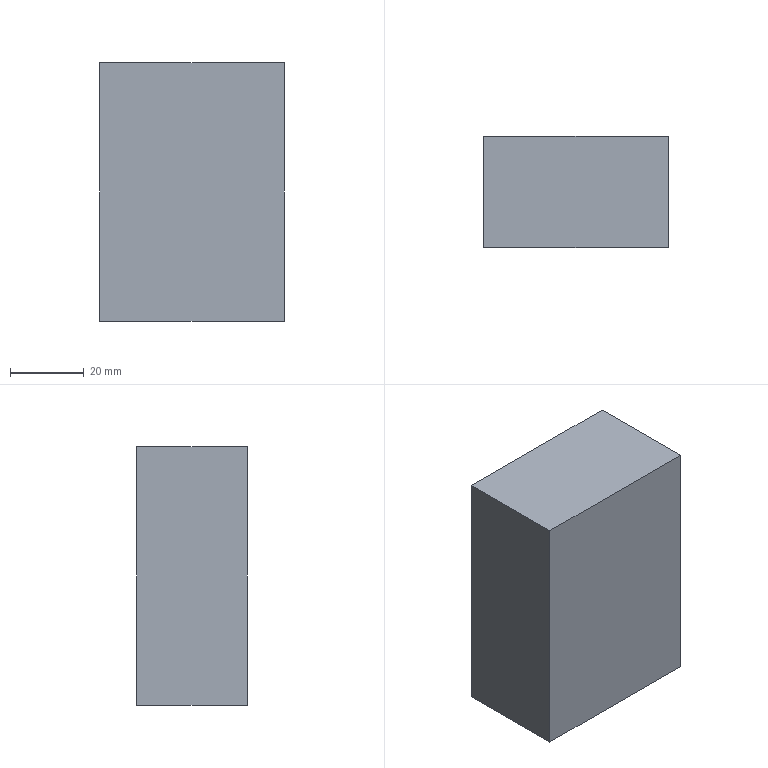Part | NX | features solid 2 | 1 solid | 10 faces | box 50 x 30 x 70 mm | volume 100916 mm3 | plane 6 | cone 2 | cylinder 2 | commonest cylinder face diameters 10 x2
STEP:
#1=CARTESIAN_POINT('',(587.5,210.,180.));
#2=VERTEX_POINT('',#1);
#3=CARTESIAN_POINT('',(582.5,210.,180.));
#4=DIRECTION('',(0.,0.,1.));
#5=DIRECTION('',(1.,0.,0.));
#6=AXIS2_PLACEMENT_3D('',#3,#4,#5);
#7=CIRCLE('',#6,5.);
#8=EDGE_CURVE('',#2,#2,#7,.T.);
#9=ORIENTED_EDGE('',*,*,#8,.F.);
#10=EDGE_LOOP('',(#9));
#11=FACE_BOUND('',#10,.T.);
#12=CARTESIAN_POINT('',(582.5,210.,183.004));
#13=VERTEX_POINT('',#12);
#14=VERTEX_LOOP('',#13);
#15=FACE_BOUND('',#14,.T.);
#16=CARTESIAN_POINT('',(582.5,210.,180.));
#17=DIRECTION('',(0.,0.,-1.));
#18=DIRECTION('',(-1.,0.,0.));
#19=AXIS2_PLACEMENT_3D('',#16,#17,#18);
#20=CONICAL_SURFACE('',#19,5.,1.03);
#21=ADVANCED_FACE('',(#11,#15),#20,.F.);
#22=CARTESIAN_POINT('',(612.5,210.,180.));
#23=VERTEX_POINT('',#22);
#24=CARTESIAN_POINT('',(607.5,210.,180.));
#25=DIRECTION('',(0.,0.,1.));
#26=DIRECTION('',(1.,0.,0.));
#27=AXIS2_PLACEMENT_3D('',#24,#25,#26);
#28=CIRCLE('',#27,5.);
#29=EDGE_CURVE('',#23,#23,#28,.T.);
#30=ORIENTED_EDGE('',*,*,#29,.F.);
#31=EDGE_LOOP('',(#30));
#32=FACE_BOUND('',#31,.T.);
#33=CARTESIAN_POINT('',(607.5,210.,183.004));
#34=VERTEX_POINT('',#33);
#35=VERTEX_LOOP('',#34);
#36=FACE_BOUND('',#35,.T.);
#37=CARTESIAN_POINT('',(607.5,210.,180.));
#38=DIRECTION('',(0.,0.,-1.));
#39=DIRECTION('',(-1.,0.,0.));
#40=AXIS2_PLACEMENT_3D('',#37,#38,#39);
#41=CONICAL_SURFACE('',#40,5.,1.03);
#42=ADVANCED_FACE('',(#32,#36),#41,.F.);
#43=ORIENTED_EDGE('',*,*,#8,.T.);
#44=EDGE_LOOP('',(#43));
#45=FACE_BOUND('',#44,.T.);
#46=CARTESIAN_POINT('',(587.5,210.,155.));
#47=VERTEX_POINT('',#46);
#48=CARTESIAN_POINT('',(582.5,210.,155.));
#49=DIRECTION('',(0.,0.,1.));
#50=DIRECTION('',(1.,0.,0.));
#51=AXIS2_PLACEMENT_3D('',#48,#49,#50);
#52=CIRCLE('',#51,5.);
#53=EDGE_CURVE('',#47,#47,#52,.T.);
#54=ORIENTED_EDGE('',*,*,#53,.F.);
#55=EDGE_LOOP('',(#54));
#56=FACE_BOUND('',#55,.T.);
#57=CARTESIAN_POINT('',(582.5,210.,155.));
#58=DIRECTION('',(0.,0.,1.));
#59=DIRECTION('',(1.,0.,0.));
#60=AXIS2_PLACEMENT_3D('',#57,#58,#59);
#61=CYLINDRICAL_SURFACE('',#60,5.);
#62=ADVANCED_FACE('',(#45,#56),#61,.F.);
#63=ORIENTED_EDGE('',*,*,#29,.T.);
#64=EDGE_LOOP('',(#63));
#65=FACE_BOUND('',#64,.T.);
#66=CARTESIAN_POINT('',(612.5,210.,155.));
#67=VERTEX_POINT('',#66);
#68=CARTESIAN_POINT('',(607.5,210.,155.));
#69=DIRECTION('',(0.,0.,1.));
#70=DIRECTION('',(1.,0.,0.));
#71=AXIS2_PLACEMENT_3D('',#68,#69,#70);
#72=CIRCLE('',#71,5.);
#73=EDGE_CURVE('',#67,#67,#72,.T.);
#74=ORIENTED_EDGE('',*,*,#73,.F.);
#75=EDGE_LOOP('',(#74));
#76=FACE_BOUND('',#75,.T.);
#77=CARTESIAN_POINT('',(607.5,210.,155.));
#78=DIRECTION('',(0.,0.,1.));
#79=DIRECTION('',(1.,0.,0.));
#80=AXIS2_PLACEMENT_3D('',#77,#78,#79);
#81=CYLINDRICAL_SURFACE('',#80,5.);
#82=ADVANCED_FACE('',(#65,#76),#81,.F.);
#83=ORIENTED_EDGE('',*,*,#73,.T.);
#84=EDGE_LOOP('',(#83));
#85=FACE_BOUND('',#84,.T.);
#86=ORIENTED_EDGE('',*,*,#53,.T.);
#87=EDGE_LOOP('',(#86));
#88=FACE_BOUND('',#87,.T.);
#89=CARTESIAN_POINT('',(570.,195.,155.));
#90=VERTEX_POINT('',#89);
#91=CARTESIAN_POINT('',(570.,225.,155.));
#92=VERTEX_POINT('',#91);
#93=CARTESIAN_POINT('',(570.,210.,155.));
#94=DIRECTION('',(0.,-1.,0.));
#95=VECTOR('',#94,1000.);
#96=LINE('',#93,#95);
#97=EDGE_CURVE('',#90,#92,#96,.F.);
#98=ORIENTED_EDGE('',*,*,#97,.T.);
#99=CARTESIAN_POINT('',(620.,225.,155.));
#100=VERTEX_POINT('',#99);
#101=CARTESIAN_POINT('',(540.,225.,155.));
#102=DIRECTION('',(1.,0.,0.));
#103=VECTOR('',#102,1000.);
#104=LINE('',#101,#103);
#105=EDGE_CURVE('',#92,#100,#104,.T.);
#106=ORIENTED_EDGE('',*,*,#105,.T.);
#107=CARTESIAN_POINT('',(620.,195.,155.));
#108=VERTEX_POINT('',#107);
#109=CARTESIAN_POINT('',(620.,210.,155.));
#110=DIRECTION('',(0.,1.,0.));
#111=VECTOR('',#110,1000.);
#112=LINE('',#109,#111);
#113=EDGE_CURVE('',#108,#100,#112,.T.);
#114=ORIENTED_EDGE('',*,*,#113,.F.);
#115=CARTESIAN_POINT('',(540.,195.,155.));
#116=DIRECTION('',(1.,0.,0.));
#117=VECTOR('',#116,1000.);
#118=LINE('',#115,#117);
#119=EDGE_CURVE('',#90,#108,#118,.T.);
#120=ORIENTED_EDGE('',*,*,#119,.F.);
#121=EDGE_LOOP('',(#98,#106,#114,#120));
#122=FACE_BOUND('',#121,.T.);
#123=CARTESIAN_POINT('',(555.,210.,155.));
#124=DIRECTION('',(0.,0.,-1.));
#125=DIRECTION('',(1.,0.,0.));
#126=AXIS2_PLACEMENT_3D('',#123,#124,#125);
#127=PLANE('',#126);
#128=ADVANCED_FACE('',(#85,#88,#122),#127,.T.);
#129=CARTESIAN_POINT('',(570.,225.,225.));
#130=VERTEX_POINT('',#129);
#131=CARTESIAN_POINT('',(570.,195.,225.));
#132=VERTEX_POINT('',#131);
#133=CARTESIAN_POINT('',(570.,210.,225.));
#134=DIRECTION('',(0.,1.,0.));
#135=VECTOR('',#134,1000.);
#136=LINE('',#133,#135);
#137=EDGE_CURVE('',#130,#132,#136,.F.);
#138=ORIENTED_EDGE('',*,*,#137,.F.);
#139=CARTESIAN_POINT('',(570.,225.,155.));
#140=DIRECTION('',(0.,0.,-1.));
#141=VECTOR('',#140,1000.);
#142=LINE('',#139,#141);
#143=EDGE_CURVE('',#92,#130,#142,.F.);
#144=ORIENTED_EDGE('',*,*,#143,.F.);
#145=ORIENTED_EDGE('',*,*,#97,.F.);
#146=CARTESIAN_POINT('',(570.,195.,155.));
#147=DIRECTION('',(0.,0.,-1.));
#148=VECTOR('',#147,1000.);
#149=LINE('',#146,#148);
#150=EDGE_CURVE('',#90,#132,#149,.F.);
#151=ORIENTED_EDGE('',*,*,#150,.T.);
#152=EDGE_LOOP('',(#138,#144,#145,#151));
#153=FACE_BOUND('',#152,.T.);
#154=CARTESIAN_POINT('',(570.,210.,130.));
#155=DIRECTION('',(1.,0.,0.));
#156=DIRECTION('',(0.,0.,1.));
#157=AXIS2_PLACEMENT_3D('',#154,#155,#156);
#158=PLANE('',#157);
#159=ADVANCED_FACE('',(#153),#158,.F.);
#160=CARTESIAN_POINT('',(620.,195.,225.));
#161=VERTEX_POINT('',#160);
#162=CARTESIAN_POINT('',(620.,195.,130.));
#163=DIRECTION('',(0.,0.,1.));
#164=VECTOR('',#163,1000.);
#165=LINE('',#162,#164);
#166=EDGE_CURVE('',#108,#161,#165,.T.);
#167=ORIENTED_EDGE('',*,*,#166,.F.);
#168=ORIENTED_EDGE('',*,*,#113,.T.);
#169=CARTESIAN_POINT('',(620.,225.,225.));
#170=VERTEX_POINT('',#169);
#171=CARTESIAN_POINT('',(620.,225.,130.));
#172=DIRECTION('',(0.,0.,1.));
#173=VECTOR('',#172,1000.);
#174=LINE('',#171,#173);
#175=EDGE_CURVE('',#100,#170,#174,.T.);
#176=ORIENTED_EDGE('',*,*,#175,.T.);
#177=CARTESIAN_POINT('',(620.,-610.,225.));
#178=DIRECTION('',(0.,1.,0.));
#179=VECTOR('',#178,1000.);
#180=LINE('',#177,#179);
#181=EDGE_CURVE('',#161,#170,#180,.T.);
#182=ORIENTED_EDGE('',*,*,#181,.F.);
#183=EDGE_LOOP('',(#167,#168,#176,#182));
#184=FACE_BOUND('',#183,.T.);
#185=CARTESIAN_POINT('',(620.,210.,130.));
#186=DIRECTION('',(1.,0.,0.));
#187=DIRECTION('',(0.,0.,1.));
#188=AXIS2_PLACEMENT_3D('',#185,#186,#187);
#189=PLANE('',#188);
#190=ADVANCED_FACE('',(#184),#189,.T.);
#191=ORIENTED_EDGE('',*,*,#166,.T.);
#192=CARTESIAN_POINT('',(500.,195.,225.));
#193=DIRECTION('',(-1.,0.,0.));
#194=VECTOR('',#193,1000.);
#195=LINE('',#192,#194);
#196=EDGE_CURVE('',#161,#132,#195,.T.);
#197=ORIENTED_EDGE('',*,*,#196,.T.);
#198=ORIENTED_EDGE('',*,*,#150,.F.);
#199=ORIENTED_EDGE('',*,*,#119,.T.);
#200=EDGE_LOOP('',(#191,#197,#198,#199));
#201=FACE_BOUND('',#200,.T.);
#202=CARTESIAN_POINT('',(500.,195.,155.));
#203=DIRECTION('',(0.,1.,0.));
#204=DIRECTION('',(0.,0.,-1.));
#205=AXIS2_PLACEMENT_3D('',#202,#203,#204);
#206=PLANE('',#205);
#207=ADVANCED_FACE('',(#201),#206,.F.);
#208=CARTESIAN_POINT('',(500.,225.,225.));
#209=DIRECTION('',(-1.,0.,0.));
#210=VECTOR('',#209,1000.);
#211=LINE('',#208,#210);
#212=EDGE_CURVE('',#170,#130,#211,.T.);
#213=ORIENTED_EDGE('',*,*,#212,.F.);
#214=ORIENTED_EDGE('',*,*,#175,.F.);
#215=ORIENTED_EDGE('',*,*,#105,.F.);
#216=ORIENTED_EDGE('',*,*,#143,.T.);
#217=EDGE_LOOP('',(#213,#214,#215,#216));
#218=FACE_BOUND('',#217,.T.);
#219=CARTESIAN_POINT('',(500.,225.,155.));
#220=DIRECTION('',(0.,1.,0.));
#221=DIRECTION('',(0.,0.,-1.));
#222=AXIS2_PLACEMENT_3D('',#219,#220,#221);
#223=PLANE('',#222);
#224=ADVANCED_FACE('',(#218),#223,.T.);
#225=ORIENTED_EDGE('',*,*,#212,.T.);
#226=ORIENTED_EDGE('',*,*,#137,.T.);
#227=ORIENTED_EDGE('',*,*,#196,.F.);
#228=ORIENTED_EDGE('',*,*,#181,.T.);
#229=EDGE_LOOP('',(#225,#226,#227,#228));
#230=FACE_BOUND('',#229,.T.);
#231=CARTESIAN_POINT('',(-620.,-610.,225.));
#232=DIRECTION('',(0.,0.,-1.));
#233=DIRECTION('',(-1.,0.,0.));
#234=AXIS2_PLACEMENT_3D('',#231,#232,#233);
#235=PLANE('',#234);
#236=ADVANCED_FACE('',(#230),#235,.F.);
#237=CLOSED_SHELL('',(#21,#42,#62,#82,#128,#159,#190,#207,#224,#236));
#238=MANIFOLD_SOLID_BREP('',#237);
#239=(LENGTH_UNIT()NAMED_UNIT(*)SI_UNIT(.MILLI.,.METRE.));
#240=UNCERTAINTY_MEASURE_WITH_UNIT(LENGTH_MEASURE(0.00001),#239,'','');
#241=(NAMED_UNIT(*)PLANE_ANGLE_UNIT()SI_UNIT($,.RADIAN.));
#242=(NAMED_UNIT(*)SI_UNIT($,.STERADIAN.)SOLID_ANGLE_UNIT());
#243=(GEOMETRIC_REPRESENTATION_CONTEXT(3)GLOBAL_UNCERTAINTY_ASSIGNED_CONTEXT((#240))GLOBAL_UNIT_ASSIGNED_CONTEXT((#239,#241,#242))REPRESENTATION_CONTEXT('',''));
#244=ADVANCED_BREP_SHAPE_REPRESENTATION('',(#238),#243);